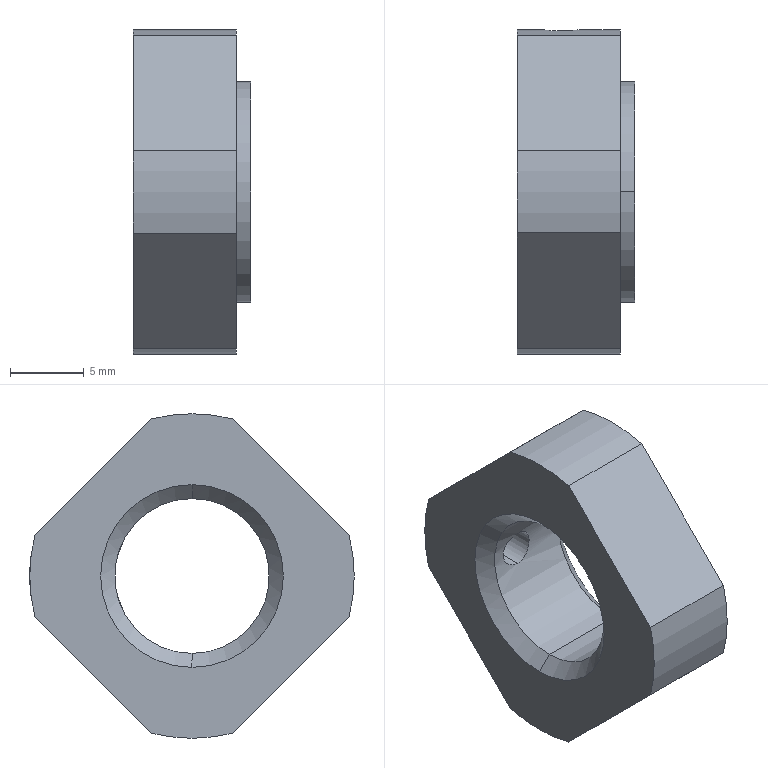Part | STEP file | 04-07 bearing retaining ring | 1 solid | 22 faces | box 8 x 22 x 22 mm | volume 1770 mm3 | cylinder 11 | plane 7 | cone 4 | commonest cylinder face diameters 22 x5 2.5 x2 10.5 x2 15 x2
STEP:
#1=CARTESIAN_POINT('',(0.947,0.,-5.25));
#2=VERTEX_POINT('',#1);
#3=CARTESIAN_POINT('',(0.947,0.,5.25));
#4=VERTEX_POINT('',#3);
#5=CARTESIAN_POINT('',(0.947,0.,0.));
#6=DIRECTION('',(-1.,0.,0.));
#7=DIRECTION('',(0.,0.,-1.));
#8=AXIS2_PLACEMENT_3D('',#5,#6,#7);
#9=CIRCLE('',#8,5.25);
#10=EDGE_CURVE('',#2,#4,#9,.T.);
#11=ORIENTED_EDGE('',*,*,#10,.F.);
#12=CARTESIAN_POINT('',(0.,0.,-6.197));
#13=VERTEX_POINT('',#12);
#14=CARTESIAN_POINT('',(0.947,0.,-5.25));
#15=DIRECTION('',(-0.7071,0.,-0.7071));
#16=VECTOR('',#15,1000.);
#17=LINE('',#14,#16);
#18=EDGE_CURVE('',#2,#13,#17,.T.);
#19=ORIENTED_EDGE('',*,*,#18,.T.);
#20=CARTESIAN_POINT('',(0.,0.,6.197));
#21=VERTEX_POINT('',#20);
#22=CARTESIAN_POINT('',(0.,0.,0.));
#23=DIRECTION('',(1.,0.,0.));
#24=DIRECTION('',(0.,0.,-1.));
#25=AXIS2_PLACEMENT_3D('',#22,#23,#24);
#26=CIRCLE('',#25,6.197);
#27=EDGE_CURVE('',#21,#13,#26,.T.);
#28=ORIENTED_EDGE('',*,*,#27,.F.);
#29=CARTESIAN_POINT('',(0.947,0.,5.25));
#30=DIRECTION('',(-0.7071,0.,0.7071));
#31=VECTOR('',#30,1000.);
#32=LINE('',#29,#31);
#33=EDGE_CURVE('',#4,#21,#32,.T.);
#34=ORIENTED_EDGE('',*,*,#33,.F.);
#35=EDGE_LOOP('',(#11,#19,#28,#34));
#36=FACE_OUTER_BOUND('',#35,.T.);
#37=CARTESIAN_POINT('',(0.947,0.,0.));
#38=DIRECTION('',(-1.,0.,0.));
#39=DIRECTION('',(0.,0.,1.));
#40=AXIS2_PLACEMENT_3D('',#37,#38,#39);
#41=CONICAL_SURFACE('',#40,5.25,0.7854);
#42=ADVANCED_FACE('',(#36),#41,.F.);
#43=CARTESIAN_POINT('',(7.053,0.,5.25));
#44=VERTEX_POINT('',#43);
#45=CARTESIAN_POINT('',(7.053,0.,-5.25));
#46=VERTEX_POINT('',#45);
#47=CARTESIAN_POINT('',(7.053,0.,0.));
#48=DIRECTION('',(1.,0.,0.));
#49=DIRECTION('',(0.,0.,-1.));
#50=AXIS2_PLACEMENT_3D('',#47,#48,#49);
#51=CIRCLE('',#50,5.25);
#52=EDGE_CURVE('',#44,#46,#51,.T.);
#53=ORIENTED_EDGE('',*,*,#52,.F.);
#54=CARTESIAN_POINT('',(8.,0.,6.197));
#55=VERTEX_POINT('',#54);
#56=CARTESIAN_POINT('',(7.053,0.,5.25));
#57=DIRECTION('',(0.7071,0.,0.7071));
#58=VECTOR('',#57,1000.);
#59=LINE('',#56,#58);
#60=EDGE_CURVE('',#44,#55,#59,.T.);
#61=ORIENTED_EDGE('',*,*,#60,.T.);
#62=CARTESIAN_POINT('',(8.,0.,-6.197));
#63=VERTEX_POINT('',#62);
#64=CARTESIAN_POINT('',(8.,0.,0.));
#65=DIRECTION('',(-1.,0.,0.));
#66=DIRECTION('',(0.,0.,-1.));
#67=AXIS2_PLACEMENT_3D('',#64,#65,#66);
#68=CIRCLE('',#67,6.197);
#69=EDGE_CURVE('',#63,#55,#68,.T.);
#70=ORIENTED_EDGE('',*,*,#69,.F.);
#71=CARTESIAN_POINT('',(7.053,0.,-5.25));
#72=DIRECTION('',(0.7071,0.,-0.7071));
#73=VECTOR('',#72,1000.);
#74=LINE('',#71,#73);
#75=EDGE_CURVE('',#46,#63,#74,.T.);
#76=ORIENTED_EDGE('',*,*,#75,.F.);
#77=EDGE_LOOP('',(#53,#61,#70,#76));
#78=FACE_OUTER_BOUND('',#77,.T.);
#79=CARTESIAN_POINT('',(7.053,0.,0.));
#80=DIRECTION('',(1.,0.,0.));
#81=DIRECTION('',(0.,0.,-1.));
#82=AXIS2_PLACEMENT_3D('',#79,#80,#81);
#83=CONICAL_SURFACE('',#82,5.25,0.7854);
#84=ADVANCED_FACE('',(#78),#83,.F.);
#85=CARTESIAN_POINT('',(3.,10.929,-1.25));
#86=VERTEX_POINT('',#85);
#87=CARTESIAN_POINT('',(3.,10.929,1.25));
#88=VERTEX_POINT('',#87);
#89=CARTESIAN_POINT('',(3.,10.929,-1.25));
#90=CARTESIAN_POINT('',(2.835,10.929,-1.25));
#91=CARTESIAN_POINT('',(2.672,10.933,-1.217));
#92=CARTESIAN_POINT('',(2.37,10.946,-1.092));
#93=CARTESIAN_POINT('',(2.231,10.955,-0.999));
#94=CARTESIAN_POINT('',(2.001,10.974,-0.7685));
#95=CARTESIAN_POINT('',(1.908,10.983,-0.6291));
#96=CARTESIAN_POINT('',(1.783,10.996,-0.3283));
#97=CARTESIAN_POINT('',(1.75,11.,-0.1637));
#98=CARTESIAN_POINT('',(1.75,11.,0.08115));
#99=CARTESIAN_POINT('',(1.758,10.999,0.164));
#100=CARTESIAN_POINT('',(1.79,10.996,0.3244));
#101=CARTESIAN_POINT('',(1.814,10.993,0.4024));
#102=CARTESIAN_POINT('',(1.908,10.983,0.6295));
#103=CARTESIAN_POINT('',(1.999,10.974,0.7671));
#104=CARTESIAN_POINT('',(2.233,10.955,1.));
#105=CARTESIAN_POINT('',(2.37,10.946,1.092));
#106=CARTESIAN_POINT('',(2.597,10.936,1.186));
#107=CARTESIAN_POINT('',(2.675,10.933,1.21));
#108=CARTESIAN_POINT('',(2.835,10.93,1.242));
#109=CARTESIAN_POINT('',(2.918,10.929,1.25));
#110=CARTESIAN_POINT('',(3.,10.929,1.25));
#111=B_SPLINE_CURVE_WITH_KNOTS('',3,(#89,#90,#91,#92,#93,#94,#95,#96,#97,#98,#99,#100,#101,#102,#103,#104,#105,#106,#107,#108,#109,#110),.UNSPECIFIED.,.F.,.F.,(4,2,2,2,2,2,2,2,2,2,4),(0.,0.0004889,0.0009778,0.001467,0.001956,0.0022,0.002445,0.002933,0.003422,0.003667,0.003911),.UNSPECIFIED.);
#112=EDGE_CURVE('',#86,#88,#111,.T.);
#113=ORIENTED_EDGE('',*,*,#112,.T.);
#114=CARTESIAN_POINT('',(3.,5.099,1.25));
#115=VERTEX_POINT('',#114);
#116=CARTESIAN_POINT('',(3.,4.702,1.25));
#117=DIRECTION('',(0.,-1.,0.));
#118=VECTOR('',#117,1000.);
#119=LINE('',#116,#118);
#120=EDGE_CURVE('',#88,#115,#119,.T.);
#121=ORIENTED_EDGE('',*,*,#120,.T.);
#122=CARTESIAN_POINT('',(3.,5.099,-1.25));
#123=VERTEX_POINT('',#122);
#124=CARTESIAN_POINT('',(3.,5.099,-1.25));
#125=CARTESIAN_POINT('',(2.834,5.099,-1.25));
#126=CARTESIAN_POINT('',(2.672,5.107,-1.217));
#127=CARTESIAN_POINT('',(2.369,5.136,-1.091));
#128=CARTESIAN_POINT('',(2.231,5.155,-0.9986));
#129=CARTESIAN_POINT('',(2.001,5.195,-0.7688));
#130=CARTESIAN_POINT('',(1.908,5.214,-0.6298));
#131=CARTESIAN_POINT('',(1.783,5.242,-0.3292));
#132=CARTESIAN_POINT('',(1.75,5.25,-0.1642));
#133=CARTESIAN_POINT('',(1.75,5.25,0.08136));
#134=CARTESIAN_POINT('',(1.758,5.248,0.1645));
#135=CARTESIAN_POINT('',(1.79,5.241,0.3251));
#136=CARTESIAN_POINT('',(1.814,5.235,0.4032));
#137=CARTESIAN_POINT('',(1.908,5.214,0.6308));
#138=CARTESIAN_POINT('',(2.,5.195,0.7682));
#139=CARTESIAN_POINT('',(2.232,5.155,1.));
#140=CARTESIAN_POINT('',(2.37,5.136,1.092));
#141=CARTESIAN_POINT('',(2.672,5.107,1.217));
#142=CARTESIAN_POINT('',(2.836,5.099,1.25));
#143=CARTESIAN_POINT('',(3.,5.099,1.25));
#144=B_SPLINE_CURVE_WITH_KNOTS('',3,(#124,#125,#126,#127,#128,#129,#130,#131,#132,#133,#134,#135,#136,#137,#138,#139,#140,#141,#142,#143),.UNSPECIFIED.,.F.,.F.,(4,2,2,2,2,2,2,2,2,4),(0.,0.0004903,0.0009805,0.001471,0.001961,0.002206,0.002451,0.002942,0.003432,0.003922),.UNSPECIFIED.);
#145=EDGE_CURVE('',#123,#115,#144,.T.);
#146=ORIENTED_EDGE('',*,*,#145,.F.);
#147=CARTESIAN_POINT('',(3.,4.702,-1.25));
#148=DIRECTION('',(0.,-1.,0.));
#149=VECTOR('',#148,1000.);
#150=LINE('',#147,#149);
#151=EDGE_CURVE('',#86,#123,#150,.T.);
#152=ORIENTED_EDGE('',*,*,#151,.F.);
#153=EDGE_LOOP('',(#113,#121,#146,#152));
#154=FACE_OUTER_BOUND('',#153,.T.);
#155=CARTESIAN_POINT('',(3.,4.702,0.));
#156=DIRECTION('',(0.,-1.,0.));
#157=DIRECTION('',(0.,0.,-1.));
#158=AXIS2_PLACEMENT_3D('',#155,#156,#157);
#159=CYLINDRICAL_SURFACE('',#158,1.25);
#160=ADVANCED_FACE('',(#154),#159,.F.);
#161=ORIENTED_EDGE('',*,*,#52,.T.);
#162=CARTESIAN_POINT('',(0.,0.,-5.25));
#163=DIRECTION('',(-1.,0.,0.));
#164=VECTOR('',#163,1000.);
#165=LINE('',#162,#164);
#166=EDGE_CURVE('',#46,#2,#165,.T.);
#167=ORIENTED_EDGE('',*,*,#166,.T.);
#168=ORIENTED_EDGE('',*,*,#10,.T.);
#169=CARTESIAN_POINT('',(0.,0.,5.25));
#170=DIRECTION('',(-1.,0.,0.));
#171=VECTOR('',#170,1000.);
#172=LINE('',#169,#171);
#173=EDGE_CURVE('',#44,#4,#172,.T.);
#174=ORIENTED_EDGE('',*,*,#173,.F.);
#175=EDGE_LOOP('',(#161,#167,#168,#174));
#176=FACE_OUTER_BOUND('',#175,.T.);
#177=CARTESIAN_POINT('',(0.,0.,0.));
#178=DIRECTION('',(-1.,0.,0.));
#179=DIRECTION('',(0.,0.,1.));
#180=AXIS2_PLACEMENT_3D('',#177,#178,#179);
#181=CYLINDRICAL_SURFACE('',#180,5.25);
#182=ADVANCED_FACE('',(#176),#181,.F.);
#183=CARTESIAN_POINT('',(7.,0.,-7.5));
#184=VERTEX_POINT('',#183);
#185=CARTESIAN_POINT('',(7.,0.,7.5));
#186=VERTEX_POINT('',#185);
#187=CARTESIAN_POINT('',(7.,0.,0.));
#188=DIRECTION('',(1.,0.,0.));
#189=DIRECTION('',(0.,0.,-1.));
#190=AXIS2_PLACEMENT_3D('',#187,#188,#189);
#191=CIRCLE('',#190,7.5);
#192=EDGE_CURVE('',#184,#186,#191,.T.);
#193=ORIENTED_EDGE('',*,*,#192,.T.);
#194=CARTESIAN_POINT('',(8.,0.,7.5));
#195=VERTEX_POINT('',#194);
#196=CARTESIAN_POINT('',(7.,0.,7.5));
#197=DIRECTION('',(1.,0.,0.));
#198=VECTOR('',#197,1000.);
#199=LINE('',#196,#198);
#200=EDGE_CURVE('',#186,#195,#199,.T.);
#201=ORIENTED_EDGE('',*,*,#200,.T.);
#202=CARTESIAN_POINT('',(8.,0.,-7.5));
#203=VERTEX_POINT('',#202);
#204=CARTESIAN_POINT('',(8.,0.,0.));
#205=DIRECTION('',(1.,0.,0.));
#206=DIRECTION('',(0.,0.,-1.));
#207=AXIS2_PLACEMENT_3D('',#204,#205,#206);
#208=CIRCLE('',#207,7.5);
#209=EDGE_CURVE('',#203,#195,#208,.T.);
#210=ORIENTED_EDGE('',*,*,#209,.F.);
#211=CARTESIAN_POINT('',(7.,0.,-7.5));
#212=DIRECTION('',(1.,0.,0.));
#213=VECTOR('',#212,1000.);
#214=LINE('',#211,#213);
#215=EDGE_CURVE('',#184,#203,#214,.T.);
#216=ORIENTED_EDGE('',*,*,#215,.F.);
#217=EDGE_LOOP('',(#193,#201,#210,#216));
#218=FACE_OUTER_BOUND('',#217,.T.);
#219=CARTESIAN_POINT('',(7.,0.,0.));
#220=DIRECTION('',(1.,0.,0.));
#221=DIRECTION('',(0.,0.,-1.));
#222=AXIS2_PLACEMENT_3D('',#219,#220,#221);
#223=CYLINDRICAL_SURFACE('',#222,7.5);
#224=ADVANCED_FACE('',(#218),#223,.T.);
#225=CARTESIAN_POINT('',(0.,-2.796,-10.639));
#226=VERTEX_POINT('',#225);
#227=CARTESIAN_POINT('',(0.,0.,-11.));
#228=VERTEX_POINT('',#227);
#229=CARTESIAN_POINT('',(0.,0.,0.));
#230=DIRECTION('',(1.,0.,0.));
#231=DIRECTION('',(0.,0.,-1.));
#232=AXIS2_PLACEMENT_3D('',#229,#230,#231);
#233=CIRCLE('',#232,11.);
#234=EDGE_CURVE('',#226,#228,#233,.T.);
#235=ORIENTED_EDGE('',*,*,#234,.T.);
#236=CARTESIAN_POINT('',(7.,0.,-11.));
#237=VERTEX_POINT('',#236);
#238=CARTESIAN_POINT('',(0.,0.,-11.));
#239=DIRECTION('',(1.,0.,0.));
#240=VECTOR('',#239,1000.);
#241=LINE('',#238,#240);
#242=EDGE_CURVE('',#228,#237,#241,.T.);
#243=ORIENTED_EDGE('',*,*,#242,.T.);
#244=CARTESIAN_POINT('',(7.,-2.796,-10.639));
#245=VERTEX_POINT('',#244);
#246=CARTESIAN_POINT('',(7.,0.,0.));
#247=DIRECTION('',(1.,0.,0.));
#248=DIRECTION('',(0.,0.,-1.));
#249=AXIS2_PLACEMENT_3D('',#246,#247,#248);
#250=CIRCLE('',#249,11.);
#251=EDGE_CURVE('',#245,#237,#250,.T.);
#252=ORIENTED_EDGE('',*,*,#251,.F.);
#253=CARTESIAN_POINT('',(0.,-2.796,-10.639));
#254=DIRECTION('',(1.,0.,0.));
#255=VECTOR('',#254,1000.);
#256=LINE('',#253,#255);
#257=EDGE_CURVE('',#226,#245,#256,.T.);
#258=ORIENTED_EDGE('',*,*,#257,.F.);
#259=EDGE_LOOP('',(#235,#243,#252,#258));
#260=FACE_OUTER_BOUND('',#259,.T.);
#261=CARTESIAN_POINT('',(0.,0.,0.));
#262=DIRECTION('',(1.,0.,0.));
#263=DIRECTION('',(0.,0.,-1.));
#264=AXIS2_PLACEMENT_3D('',#261,#262,#263);
#265=CYLINDRICAL_SURFACE('',#264,11.);
#266=ADVANCED_FACE('',(#260),#265,.T.);
#267=ORIENTED_EDGE('',*,*,#112,.F.);
#268=CARTESIAN_POINT('',(3.,10.929,1.25));
#269=CARTESIAN_POINT('',(3.163,10.929,1.25));
#270=CARTESIAN_POINT('',(3.328,10.933,1.217));
#271=CARTESIAN_POINT('',(3.629,10.946,1.093));
#272=CARTESIAN_POINT('',(3.768,10.955,0.9996));
#273=CARTESIAN_POINT('',(3.999,10.974,0.7693));
#274=CARTESIAN_POINT('',(4.091,10.983,0.6309));
#275=CARTESIAN_POINT('',(4.217,10.996,0.3283));
#276=CARTESIAN_POINT('',(4.25,11.,0.1662));
#277=CARTESIAN_POINT('',(4.25,11.,-0.1643));
#278=CARTESIAN_POINT('',(4.218,10.996,-0.3266));
#279=CARTESIAN_POINT('',(4.092,10.983,-0.6294));
#280=CARTESIAN_POINT('',(4.,10.974,-0.768));
#281=CARTESIAN_POINT('',(3.769,10.955,-0.9986));
#282=CARTESIAN_POINT('',(3.63,10.946,-1.092));
#283=CARTESIAN_POINT('',(3.329,10.933,-1.217));
#284=CARTESIAN_POINT('',(3.165,10.929,-1.25));
#285=CARTESIAN_POINT('',(3.,10.929,-1.25));
#286=B_SPLINE_CURVE_WITH_KNOTS('',3,(#268,#269,#270,#271,#272,#273,#274,#275,#276,#277,#278,#279,#280,#281,#282,#283,#284,#285),.UNSPECIFIED.,.F.,.F.,(4,2,2,2,2,2,2,2,4),(0.003911,0.0044,0.004889,0.005378,0.005866,0.006355,0.006844,0.007333,0.007822),.UNSPECIFIED.);
#287=EDGE_CURVE('',#88,#86,#286,.T.);
#288=ORIENTED_EDGE('',*,*,#287,.F.);
#289=EDGE_LOOP('',(#267,#288));
#290=FACE_BOUND('',#289,.T.);
#291=CARTESIAN_POINT('',(7.,10.639,-2.796));
#292=VERTEX_POINT('',#291);
#293=CARTESIAN_POINT('',(7.,10.639,2.796));
#294=VERTEX_POINT('',#293);
#295=CARTESIAN_POINT('',(7.,0.,0.));
#296=DIRECTION('',(1.,0.,0.));
#297=DIRECTION('',(0.,0.,-1.));
#298=AXIS2_PLACEMENT_3D('',#295,#296,#297);
#299=CIRCLE('',#298,11.);
#300=EDGE_CURVE('',#292,#294,#299,.T.);
#301=ORIENTED_EDGE('',*,*,#300,.F.);
#302=CARTESIAN_POINT('',(0.,10.639,-2.796));
#303=VERTEX_POINT('',#302);
#304=CARTESIAN_POINT('',(0.,10.639,-2.796));
#305=DIRECTION('',(1.,0.,0.));
#306=VECTOR('',#305,1000.);
#307=LINE('',#304,#306);
#308=EDGE_CURVE('',#303,#292,#307,.T.);
#309=ORIENTED_EDGE('',*,*,#308,.F.);
#310=CARTESIAN_POINT('',(0.,10.639,2.796));
#311=VERTEX_POINT('',#310);
#312=CARTESIAN_POINT('',(0.,0.,0.));
#313=DIRECTION('',(1.,0.,0.));
#314=DIRECTION('',(0.,0.,-1.));
#315=AXIS2_PLACEMENT_3D('',#312,#313,#314);
#316=CIRCLE('',#315,11.);
#317=EDGE_CURVE('',#303,#311,#316,.T.);
#318=ORIENTED_EDGE('',*,*,#317,.T.);
#319=CARTESIAN_POINT('',(0.,10.639,2.796));
#320=DIRECTION('',(1.,0.,0.));
#321=VECTOR('',#320,1000.);
#322=LINE('',#319,#321);
#323=EDGE_CURVE('',#311,#294,#322,.T.);
#324=ORIENTED_EDGE('',*,*,#323,.T.);
#325=EDGE_LOOP('',(#301,#309,#318,#324));
#326=FACE_OUTER_BOUND('',#325,.T.);
#327=CARTESIAN_POINT('',(0.,0.,0.));
#328=DIRECTION('',(1.,0.,0.));
#329=DIRECTION('',(0.,0.,-1.));
#330=AXIS2_PLACEMENT_3D('',#327,#328,#329);
#331=CYLINDRICAL_SURFACE('',#330,11.);
#332=ADVANCED_FACE('',(#290,#326),#331,.T.);
#333=CARTESIAN_POINT('',(7.,2.796,-10.639));
#334=VERTEX_POINT('',#333);
#335=CARTESIAN_POINT('',(7.,2.796,-10.639));
#336=DIRECTION('',(0.,0.7071,0.7071));
#337=VECTOR('',#336,1000.);
#338=LINE('',#335,#337);
#339=EDGE_CURVE('',#334,#292,#338,.T.);
#340=ORIENTED_EDGE('',*,*,#339,.F.);
#341=CARTESIAN_POINT('',(0.,2.796,-10.639));
#342=VERTEX_POINT('',#341);
#343=CARTESIAN_POINT('',(0.,2.796,-10.639));
#344=DIRECTION('',(1.,0.,0.));
#345=VECTOR('',#344,1000.);
#346=LINE('',#343,#345);
#347=EDGE_CURVE('',#342,#334,#346,.T.);
#348=ORIENTED_EDGE('',*,*,#347,.F.);
#349=CARTESIAN_POINT('',(0.,2.796,-10.639));
#350=DIRECTION('',(0.,0.7071,0.7071));
#351=VECTOR('',#350,1000.);
#352=LINE('',#349,#351);
#353=EDGE_CURVE('',#342,#303,#352,.T.);
#354=ORIENTED_EDGE('',*,*,#353,.T.);
#355=ORIENTED_EDGE('',*,*,#308,.T.);
#356=EDGE_LOOP('',(#340,#348,#354,#355));
#357=FACE_OUTER_BOUND('',#356,.T.);
#358=CARTESIAN_POINT('',(0.,2.796,-10.639));
#359=DIRECTION('',(0.,0.7071,-0.7071));
#360=DIRECTION('',(0.,0.7071,0.7071));
#361=AXIS2_PLACEMENT_3D('',#358,#359,#360);
#362=PLANE('',#361);
#363=ADVANCED_FACE('',(#357),#362,.T.);
#364=ORIENTED_EDGE('',*,*,#242,.F.);
#365=CARTESIAN_POINT('',(0.,0.,0.));
#366=DIRECTION('',(1.,0.,0.));
#367=DIRECTION('',(0.,0.,-1.));
#368=AXIS2_PLACEMENT_3D('',#365,#366,#367);
#369=CIRCLE('',#368,11.);
#370=EDGE_CURVE('',#228,#342,#369,.T.);
#371=ORIENTED_EDGE('',*,*,#370,.T.);
#372=ORIENTED_EDGE('',*,*,#347,.T.);
#373=CARTESIAN_POINT('',(7.,0.,0.));
#374=DIRECTION('',(1.,0.,0.));
#375=DIRECTION('',(0.,0.,-1.));
#376=AXIS2_PLACEMENT_3D('',#373,#374,#375);
#377=CIRCLE('',#376,11.);
#378=EDGE_CURVE('',#237,#334,#377,.T.);
#379=ORIENTED_EDGE('',*,*,#378,.F.);
#380=EDGE_LOOP('',(#364,#371,#372,#379));
#381=FACE_OUTER_BOUND('',#380,.T.);
#382=CARTESIAN_POINT('',(0.,0.,0.));
#383=DIRECTION('',(1.,0.,0.));
#384=DIRECTION('',(0.,0.,-1.));
#385=AXIS2_PLACEMENT_3D('',#382,#383,#384);
#386=CYLINDRICAL_SURFACE('',#385,11.);
#387=ADVANCED_FACE('',(#381),#386,.T.);
#388=CARTESIAN_POINT('',(7.,-10.639,-2.796));
#389=VERTEX_POINT('',#388);
#390=CARTESIAN_POINT('',(7.,-10.639,-2.796));
#391=DIRECTION('',(0.,0.7071,-0.7071));
#392=VECTOR('',#391,1000.);
#393=LINE('',#390,#392);
#394=EDGE_CURVE('',#389,#245,#393,.T.);
#395=ORIENTED_EDGE('',*,*,#394,.F.);
#396=CARTESIAN_POINT('',(0.,-10.639,-2.796));
#397=VERTEX_POINT('',#396);
#398=CARTESIAN_POINT('',(0.,-10.639,-2.796));
#399=DIRECTION('',(1.,0.,0.));
#400=VECTOR('',#399,1000.);
#401=LINE('',#398,#400);
#402=EDGE_CURVE('',#397,#389,#401,.T.);
#403=ORIENTED_EDGE('',*,*,#402,.F.);
#404=CARTESIAN_POINT('',(0.,-10.639,-2.796));
#405=DIRECTION('',(0.,0.7071,-0.7071));
#406=VECTOR('',#405,1000.);
#407=LINE('',#404,#406);
#408=EDGE_CURVE('',#397,#226,#407,.T.);
#409=ORIENTED_EDGE('',*,*,#408,.T.);
#410=ORIENTED_EDGE('',*,*,#257,.T.);
#411=EDGE_LOOP('',(#395,#403,#409,#410));
#412=FACE_OUTER_BOUND('',#411,.T.);
#413=CARTESIAN_POINT('',(0.,-10.639,-2.796));
#414=DIRECTION('',(0.,-0.7071,-0.7071));
#415=DIRECTION('',(0.,0.7071,-0.7071));
#416=AXIS2_PLACEMENT_3D('',#413,#414,#415);
#417=PLANE('',#416);
#418=ADVANCED_FACE('',(#412),#417,.T.);
#419=CARTESIAN_POINT('',(7.,-10.639,2.796));
#420=VERTEX_POINT('',#419);
#421=CARTESIAN_POINT('',(7.,0.,0.));
#422=DIRECTION('',(1.,0.,0.));
#423=DIRECTION('',(0.,0.,-1.));
#424=AXIS2_PLACEMENT_3D('',#421,#422,#423);
#425=CIRCLE('',#424,11.);
#426=EDGE_CURVE('',#420,#389,#425,.T.);
#427=ORIENTED_EDGE('',*,*,#426,.F.);
#428=CARTESIAN_POINT('',(0.,-10.639,2.796));
#429=VERTEX_POINT('',#428);
#430=CARTESIAN_POINT('',(0.,-10.639,2.796));
#431=DIRECTION('',(1.,0.,0.));
#432=VECTOR('',#431,1000.);
#433=LINE('',#430,#432);
#434=EDGE_CURVE('',#429,#420,#433,.T.);
#435=ORIENTED_EDGE('',*,*,#434,.F.);
#436=CARTESIAN_POINT('',(0.,0.,0.));
#437=DIRECTION('',(1.,0.,0.));
#438=DIRECTION('',(0.,0.,-1.));
#439=AXIS2_PLACEMENT_3D('',#436,#437,#438);
#440=CIRCLE('',#439,11.);
#441=EDGE_CURVE('',#429,#397,#440,.T.);
#442=ORIENTED_EDGE('',*,*,#441,.T.);
#443=ORIENTED_EDGE('',*,*,#402,.T.);
#444=EDGE_LOOP('',(#427,#435,#442,#443));
#445=FACE_OUTER_BOUND('',#444,.T.);
#446=CARTESIAN_POINT('',(0.,0.,0.));
#447=DIRECTION('',(1.,0.,0.));
#448=DIRECTION('',(0.,0.,-1.));
#449=AXIS2_PLACEMENT_3D('',#446,#447,#448);
#450=CYLINDRICAL_SURFACE('',#449,11.);
#451=ADVANCED_FACE('',(#445),#450,.T.);
#452=CARTESIAN_POINT('',(7.,-2.796,10.639));
#453=VERTEX_POINT('',#452);
#454=CARTESIAN_POINT('',(7.,-2.796,10.639));
#455=DIRECTION('',(0.,-0.7071,-0.7071));
#456=VECTOR('',#455,1000.);
#457=LINE('',#454,#456);
#458=EDGE_CURVE('',#453,#420,#457,.T.);
#459=ORIENTED_EDGE('',*,*,#458,.F.);
#460=CARTESIAN_POINT('',(0.,-2.796,10.639));
#461=VERTEX_POINT('',#460);
#462=CARTESIAN_POINT('',(0.,-2.796,10.639));
#463=DIRECTION('',(1.,0.,0.));
#464=VECTOR('',#463,1000.);
#465=LINE('',#462,#464);
#466=EDGE_CURVE('',#461,#453,#465,.T.);
#467=ORIENTED_EDGE('',*,*,#466,.F.);
#468=CARTESIAN_POINT('',(0.,-2.796,10.639));
#469=DIRECTION('',(0.,-0.7071,-0.7071));
#470=VECTOR('',#469,1000.);
#471=LINE('',#468,#470);
#472=EDGE_CURVE('',#461,#429,#471,.T.);
#473=ORIENTED_EDGE('',*,*,#472,.T.);
#474=ORIENTED_EDGE('',*,*,#434,.T.);
#475=EDGE_LOOP('',(#459,#467,#473,#474));
#476=FACE_OUTER_BOUND('',#475,.T.);
#477=CARTESIAN_POINT('',(0.,-2.796,10.639));
#478=DIRECTION('',(0.,-0.7071,0.7071));
#479=DIRECTION('',(0.,-0.7071,-0.7071));
#480=AXIS2_PLACEMENT_3D('',#477,#478,#479);
#481=PLANE('',#480);
#482=ADVANCED_FACE('',(#476),#481,.T.);
#483=CARTESIAN_POINT('',(7.,2.796,10.639));
#484=VERTEX_POINT('',#483);
#485=CARTESIAN_POINT('',(7.,0.,0.));
#486=DIRECTION('',(1.,0.,0.));
#487=DIRECTION('',(0.,0.,-1.));
#488=AXIS2_PLACEMENT_3D('',#485,#486,#487);
#489=CIRCLE('',#488,11.);
#490=EDGE_CURVE('',#484,#453,#489,.T.);
#491=ORIENTED_EDGE('',*,*,#490,.F.);
#492=CARTESIAN_POINT('',(0.,2.796,10.639));
#493=VERTEX_POINT('',#492);
#494=CARTESIAN_POINT('',(0.,2.796,10.639));
#495=DIRECTION('',(1.,0.,0.));
#496=VECTOR('',#495,1000.);
#497=LINE('',#494,#496);
#498=EDGE_CURVE('',#493,#484,#497,.T.);
#499=ORIENTED_EDGE('',*,*,#498,.F.);
#500=CARTESIAN_POINT('',(0.,0.,0.));
#501=DIRECTION('',(1.,0.,0.));
#502=DIRECTION('',(0.,0.,-1.));
#503=AXIS2_PLACEMENT_3D('',#500,#501,#502);
#504=CIRCLE('',#503,11.);
#505=EDGE_CURVE('',#493,#461,#504,.T.);
#506=ORIENTED_EDGE('',*,*,#505,.T.);
#507=ORIENTED_EDGE('',*,*,#466,.T.);
#508=EDGE_LOOP('',(#491,#499,#506,#507));
#509=FACE_OUTER_BOUND('',#508,.T.);
#510=CARTESIAN_POINT('',(0.,0.,0.));
#511=DIRECTION('',(1.,0.,0.));
#512=DIRECTION('',(0.,0.,-1.));
#513=AXIS2_PLACEMENT_3D('',#510,#511,#512);
#514=CYLINDRICAL_SURFACE('',#513,11.);
#515=ADVANCED_FACE('',(#509),#514,.T.);
#516=CARTESIAN_POINT('',(7.,10.639,2.796));
#517=DIRECTION('',(0.,-0.7071,0.7071));
#518=VECTOR('',#517,1000.);
#519=LINE('',#516,#518);
#520=EDGE_CURVE('',#294,#484,#519,.T.);
#521=ORIENTED_EDGE('',*,*,#520,.F.);
#522=ORIENTED_EDGE('',*,*,#323,.F.);
#523=CARTESIAN_POINT('',(0.,10.639,2.796));
#524=DIRECTION('',(0.,-0.7071,0.7071));
#525=VECTOR('',#524,1000.);
#526=LINE('',#523,#525);
#527=EDGE_CURVE('',#311,#493,#526,.T.);
#528=ORIENTED_EDGE('',*,*,#527,.T.);
#529=ORIENTED_EDGE('',*,*,#498,.T.);
#530=EDGE_LOOP('',(#521,#522,#528,#529));
#531=FACE_OUTER_BOUND('',#530,.T.);
#532=CARTESIAN_POINT('',(0.,10.639,2.796));
#533=DIRECTION('',(0.,0.7071,0.7071));
#534=DIRECTION('',(0.,-0.7071,0.7071));
#535=AXIS2_PLACEMENT_3D('',#532,#533,#534);
#536=PLANE('',#535);
#537=ADVANCED_FACE('',(#531),#536,.T.);
#538=ORIENTED_EDGE('',*,*,#27,.T.);
#539=CARTESIAN_POINT('',(0.,0.,0.));
#540=DIRECTION('',(1.,0.,0.));
#541=DIRECTION('',(0.,0.,-1.));
#542=AXIS2_PLACEMENT_3D('',#539,#540,#541);
#543=CIRCLE('',#542,6.197);
#544=EDGE_CURVE('',#13,#21,#543,.T.);
#545=ORIENTED_EDGE('',*,*,#544,.T.);
#546=EDGE_LOOP('',(#538,#545));
#547=FACE_BOUND('',#546,.T.);
#548=ORIENTED_EDGE('',*,*,#317,.F.);
#549=ORIENTED_EDGE('',*,*,#353,.F.);
#550=ORIENTED_EDGE('',*,*,#370,.F.);
#551=ORIENTED_EDGE('',*,*,#234,.F.);
#552=ORIENTED_EDGE('',*,*,#408,.F.);
#553=ORIENTED_EDGE('',*,*,#441,.F.);
#554=ORIENTED_EDGE('',*,*,#472,.F.);
#555=ORIENTED_EDGE('',*,*,#505,.F.);
#556=ORIENTED_EDGE('',*,*,#527,.F.);
#557=EDGE_LOOP('',(#548,#549,#550,#551,#552,#553,#554,#555,#556));
#558=FACE_OUTER_BOUND('',#557,.T.);
#559=CARTESIAN_POINT('',(0.,0.,0.));
#560=DIRECTION('',(1.,0.,0.));
#561=DIRECTION('',(0.,0.,-1.));
#562=AXIS2_PLACEMENT_3D('',#559,#560,#561);
#563=PLANE('',#562);
#564=ADVANCED_FACE('',(#547,#558),#563,.F.);
#565=ORIENTED_EDGE('',*,*,#192,.F.);
#566=CARTESIAN_POINT('',(7.,0.,0.));
#567=DIRECTION('',(1.,0.,0.));
#568=DIRECTION('',(0.,0.,-1.));
#569=AXIS2_PLACEMENT_3D('',#566,#567,#568);
#570=CIRCLE('',#569,7.5);
#571=EDGE_CURVE('',#186,#184,#570,.T.);
#572=ORIENTED_EDGE('',*,*,#571,.F.);
#573=EDGE_LOOP('',(#565,#572));
#574=FACE_BOUND('',#573,.T.);
#575=ORIENTED_EDGE('',*,*,#300,.T.);
#576=ORIENTED_EDGE('',*,*,#520,.T.);
#577=ORIENTED_EDGE('',*,*,#490,.T.);
#578=ORIENTED_EDGE('',*,*,#458,.T.);
#579=ORIENTED_EDGE('',*,*,#426,.T.);
#580=ORIENTED_EDGE('',*,*,#394,.T.);
#581=ORIENTED_EDGE('',*,*,#251,.T.);
#582=ORIENTED_EDGE('',*,*,#378,.T.);
#583=ORIENTED_EDGE('',*,*,#339,.T.);
#584=EDGE_LOOP('',(#575,#576,#577,#578,#579,#580,#581,#582,#583));
#585=FACE_OUTER_BOUND('',#584,.T.);
#586=CARTESIAN_POINT('',(7.,0.,0.));
#587=DIRECTION('',(1.,0.,0.));
#588=DIRECTION('',(0.,0.,-1.));
#589=AXIS2_PLACEMENT_3D('',#586,#587,#588);
#590=PLANE('',#589);
#591=ADVANCED_FACE('',(#574,#585),#590,.T.);
#592=ORIENTED_EDGE('',*,*,#200,.F.);
#593=ORIENTED_EDGE('',*,*,#571,.T.);
#594=ORIENTED_EDGE('',*,*,#215,.T.);
#595=CARTESIAN_POINT('',(8.,0.,0.));
#596=DIRECTION('',(1.,0.,0.));
#597=DIRECTION('',(0.,0.,-1.));
#598=AXIS2_PLACEMENT_3D('',#595,#596,#597);
#599=CIRCLE('',#598,7.5);
#600=EDGE_CURVE('',#195,#203,#599,.T.);
#601=ORIENTED_EDGE('',*,*,#600,.F.);
#602=EDGE_LOOP('',(#592,#593,#594,#601));
#603=FACE_OUTER_BOUND('',#602,.T.);
#604=CARTESIAN_POINT('',(7.,0.,0.));
#605=DIRECTION('',(1.,0.,0.));
#606=DIRECTION('',(0.,0.,-1.));
#607=AXIS2_PLACEMENT_3D('',#604,#605,#606);
#608=CYLINDRICAL_SURFACE('',#607,7.5);
#609=ADVANCED_FACE('',(#603),#608,.T.);
#610=ORIENTED_EDGE('',*,*,#69,.T.);
#611=CARTESIAN_POINT('',(8.,0.,0.));
#612=DIRECTION('',(-1.,0.,0.));
#613=DIRECTION('',(0.,0.,-1.));
#614=AXIS2_PLACEMENT_3D('',#611,#612,#613);
#615=CIRCLE('',#614,6.197);
#616=EDGE_CURVE('',#55,#63,#615,.T.);
#617=ORIENTED_EDGE('',*,*,#616,.T.);
#618=EDGE_LOOP('',(#610,#617));
#619=FACE_BOUND('',#618,.T.);
#620=ORIENTED_EDGE('',*,*,#209,.T.);
#621=ORIENTED_EDGE('',*,*,#600,.T.);
#622=EDGE_LOOP('',(#620,#621));
#623=FACE_OUTER_BOUND('',#622,.T.);
#624=CARTESIAN_POINT('',(8.,0.,0.));
#625=DIRECTION('',(1.,0.,0.));
#626=DIRECTION('',(0.,0.,-1.));
#627=AXIS2_PLACEMENT_3D('',#624,#625,#626);
#628=PLANE('',#627);
#629=ADVANCED_FACE('',(#619,#623),#628,.T.);
#630=ORIENTED_EDGE('',*,*,#166,.F.);
#631=CARTESIAN_POINT('',(7.053,0.,0.));
#632=DIRECTION('',(1.,0.,0.));
#633=DIRECTION('',(0.,0.,-1.));
#634=AXIS2_PLACEMENT_3D('',#631,#632,#633);
#635=CIRCLE('',#634,5.25);
#636=EDGE_CURVE('',#46,#44,#635,.T.);
#637=ORIENTED_EDGE('',*,*,#636,.T.);
#638=ORIENTED_EDGE('',*,*,#173,.T.);
#639=CARTESIAN_POINT('',(0.947,0.,0.));
#640=DIRECTION('',(-1.,0.,0.));
#641=DIRECTION('',(0.,0.,-1.));
#642=AXIS2_PLACEMENT_3D('',#639,#640,#641);
#643=CIRCLE('',#642,5.25);
#644=EDGE_CURVE('',#4,#2,#643,.T.);
#645=ORIENTED_EDGE('',*,*,#644,.T.);
#646=EDGE_LOOP('',(#630,#637,#638,#645));
#647=FACE_OUTER_BOUND('',#646,.T.);
#648=ORIENTED_EDGE('',*,*,#145,.T.);
#649=CARTESIAN_POINT('',(3.,5.099,1.25));
#650=CARTESIAN_POINT('',(3.163,5.099,1.25));
#651=CARTESIAN_POINT('',(3.328,5.107,1.217));
#652=CARTESIAN_POINT('',(3.63,5.136,1.092));
#653=CARTESIAN_POINT('',(3.768,5.155,0.9995));
#654=CARTESIAN_POINT('',(3.999,5.195,0.7692));
#655=CARTESIAN_POINT('',(4.091,5.214,0.632));
#656=CARTESIAN_POINT('',(4.217,5.242,0.3281));
#657=CARTESIAN_POINT('',(4.25,5.25,0.1654));
#658=CARTESIAN_POINT('',(4.25,5.25,-0.08202));
#659=CARTESIAN_POINT('',(4.242,5.248,-0.1634));
#660=CARTESIAN_POINT('',(4.21,5.241,-0.3238));
#661=CARTESIAN_POINT('',(4.186,5.235,-0.4036));
#662=CARTESIAN_POINT('',(4.092,5.214,-0.6298));
#663=CARTESIAN_POINT('',(3.999,5.195,-0.7686));
#664=CARTESIAN_POINT('',(3.77,5.156,-0.9982));
#665=CARTESIAN_POINT('',(3.631,5.136,-1.091));
#666=CARTESIAN_POINT('',(3.33,5.108,-1.217));
#667=CARTESIAN_POINT('',(3.166,5.099,-1.25));
#668=CARTESIAN_POINT('',(3.,5.099,-1.25));
#669=B_SPLINE_CURVE_WITH_KNOTS('',3,(#649,#650,#651,#652,#653,#654,#655,#656,#657,#658,#659,#660,#661,#662,#663,#664,#665,#666,#667,#668),.UNSPECIFIED.,.F.,.F.,(4,2,2,2,2,2,2,2,2,4),(0.003922,0.004412,0.004902,0.005393,0.005883,0.006128,0.006373,0.006863,0.007353,0.007843),.UNSPECIFIED.);
#670=EDGE_CURVE('',#115,#123,#669,.T.);
#671=ORIENTED_EDGE('',*,*,#670,.T.);
#672=EDGE_LOOP('',(#648,#671));
#673=FACE_BOUND('',#672,.T.);
#674=CARTESIAN_POINT('',(0.,0.,0.));
#675=DIRECTION('',(-1.,0.,0.));
#676=DIRECTION('',(0.,0.,1.));
#677=AXIS2_PLACEMENT_3D('',#674,#675,#676);
#678=CYLINDRICAL_SURFACE('',#677,5.25);
#679=ADVANCED_FACE('',(#647,#673),#678,.F.);
#680=ORIENTED_EDGE('',*,*,#120,.F.);
#681=ORIENTED_EDGE('',*,*,#287,.T.);
#682=ORIENTED_EDGE('',*,*,#151,.T.);
#683=ORIENTED_EDGE('',*,*,#670,.F.);
#684=EDGE_LOOP('',(#680,#681,#682,#683));
#685=FACE_OUTER_BOUND('',#684,.T.);
#686=CARTESIAN_POINT('',(3.,4.702,0.));
#687=DIRECTION('',(0.,-1.,0.));
#688=DIRECTION('',(0.,0.,-1.));
#689=AXIS2_PLACEMENT_3D('',#686,#687,#688);
#690=CYLINDRICAL_SURFACE('',#689,1.25);
#691=ADVANCED_FACE('',(#685),#690,.F.);
#692=ORIENTED_EDGE('',*,*,#60,.F.);
#693=ORIENTED_EDGE('',*,*,#636,.F.);
#694=ORIENTED_EDGE('',*,*,#75,.T.);
#695=ORIENTED_EDGE('',*,*,#616,.F.);
#696=EDGE_LOOP('',(#692,#693,#694,#695));
#697=FACE_OUTER_BOUND('',#696,.T.);
#698=CARTESIAN_POINT('',(7.053,0.,0.));
#699=DIRECTION('',(1.,0.,0.));
#700=DIRECTION('',(0.,0.,-1.));
#701=AXIS2_PLACEMENT_3D('',#698,#699,#700);
#702=CONICAL_SURFACE('',#701,5.25,0.7854);
#703=ADVANCED_FACE('',(#697),#702,.F.);
#704=ORIENTED_EDGE('',*,*,#18,.F.);
#705=ORIENTED_EDGE('',*,*,#644,.F.);
#706=ORIENTED_EDGE('',*,*,#33,.T.);
#707=ORIENTED_EDGE('',*,*,#544,.F.);
#708=EDGE_LOOP('',(#704,#705,#706,#707));
#709=FACE_OUTER_BOUND('',#708,.T.);
#710=CARTESIAN_POINT('',(0.947,0.,0.));
#711=DIRECTION('',(-1.,0.,0.));
#712=DIRECTION('',(0.,0.,1.));
#713=AXIS2_PLACEMENT_3D('',#710,#711,#712);
#714=CONICAL_SURFACE('',#713,5.25,0.7854);
#715=ADVANCED_FACE('',(#709),#714,.F.);
#716=CLOSED_SHELL('',(#42,#84,#160,#182,#224,#266,#332,#363,#387,#418,#451,#482,#515,#537,#564,#591,#609,#629,#679,#691,#703,#715));
#717=MANIFOLD_SOLID_BREP('',#716);
#718=CARTESIAN_POINT('',(0.,0.,0.));
#719=DIRECTION('',(0.,0.,1.));
#720=DIRECTION('',(1.,0.,0.));
#721=AXIS2_PLACEMENT_3D('',#718,#719,#720);
#722=(LENGTH_UNIT()NAMED_UNIT(*)SI_UNIT(.MILLI.,.METRE.));
#723=UNCERTAINTY_MEASURE_WITH_UNIT(LENGTH_MEASURE(0.00001),#722,'','');
#724=(NAMED_UNIT(*)PLANE_ANGLE_UNIT()SI_UNIT($,.RADIAN.));
#725=(NAMED_UNIT(*)SI_UNIT($,.STERADIAN.)SOLID_ANGLE_UNIT());
#726=(GEOMETRIC_REPRESENTATION_CONTEXT(3)GLOBAL_UNCERTAINTY_ASSIGNED_CONTEXT((#723))GLOBAL_UNIT_ASSIGNED_CONTEXT((#722,#724,#725))REPRESENTATION_CONTEXT('',''));
#727=ADVANCED_BREP_SHAPE_REPRESENTATION('',(#717,#721),#726);